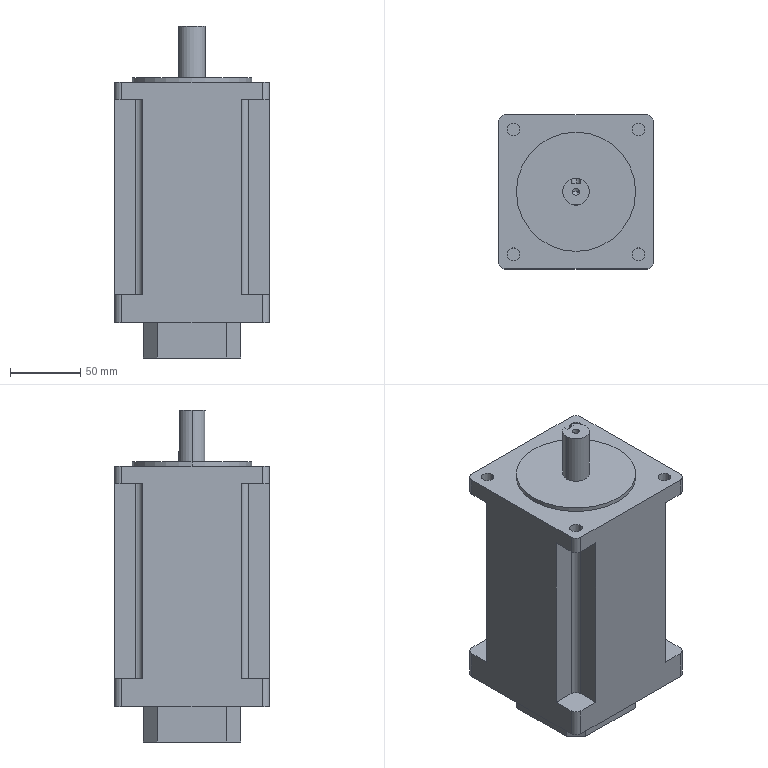Part | SolidWorks | features ICE 5, Fillet 3, HoleWzd 2, Chamfer 1, CirPattern 1, Extrusion 1 | 1 solid | 66 faces | box 110 x 110 x 236.5 mm | volume 1994232 mm3 | plane 36 | cylinder 28 | cone 2 | commonest cylinder face diameters 10 x12 9 x8 5 x2 6 x2 19 x2 85 x2